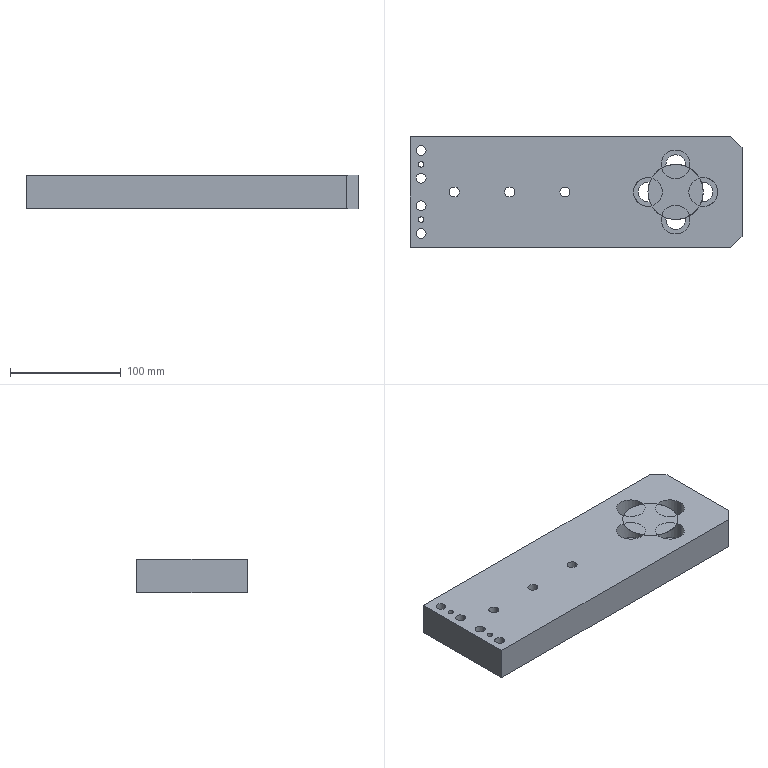Part | NX | features BREP 1 | 1 solid | 74 faces | box 300 x 100 x 30.1 mm | volume 827704 mm3 | cylinder 50 | plane 24 | commonest cylinder face diameters 9 x14 15 x14 17.5 x8 26 x8 5 x4 50 x2